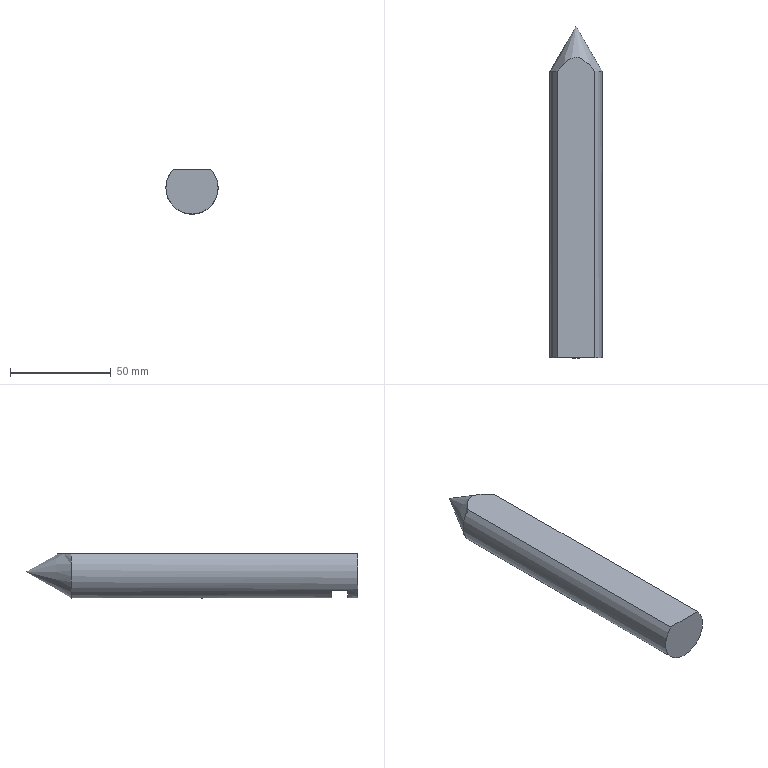Part | NX | features EXTRUDE 4, DATUM_CSYS 2, CONE 1, DATUM_PLANE 1, RECT_SLOT 1, SKETCH 1 | 1 solid | 12 faces | box 26 x 165 x 22 mm | volume 69817 mm3 | plane 7 | cylinder 4 | cone 1 | commonest cylinder face diameters 5 x2 26 x1 32 x1
STEP:
#1=CARTESIAN_POINT('',(-9.381,142.483,9.));
#2=VERTEX_POINT('',#1);
#3=CARTESIAN_POINT('',(0.06208,142.483,-13.));
#4=VERTEX_POINT('',#3);
#5=CARTESIAN_POINT('',(0.,142.483,0.));
#6=DIRECTION('',(0.,-1.,0.));
#7=DIRECTION('',(0.,0.,-1.));
#8=AXIS2_PLACEMENT_3D('',#5,#6,#7);
#9=CIRCLE('',#8,13.);
#10=EDGE_CURVE('',#2,#4,#9,.T.);
#11=ORIENTED_EDGE('',*,*,#10,.T.);
#12=CARTESIAN_POINT('',(-2.438,139.983,-12.769));
#13=VERTEX_POINT('',#12);
#14=CARTESIAN_POINT('',(0.06208,142.483,-13.));
#15=CARTESIAN_POINT('',(-0.5912,142.483,-13.003));
#16=CARTESIAN_POINT('',(-1.896,141.938,-12.889));
#17=CARTESIAN_POINT('',(-2.438,140.645,-12.769));
#18=CARTESIAN_POINT('',(-2.438,139.983,-12.769));
#19=B_SPLINE_CURVE_WITH_KNOTS('',3,(#14,#15,#16,#17,#18),.UNSPECIFIED.,.F.,.F.,(4,1,4),(0.003919,0.005876,0.007832),.UNSPECIFIED.);
#20=EDGE_CURVE('',#4,#13,#19,.T.);
#21=ORIENTED_EDGE('',*,*,#20,.T.);
#22=CARTESIAN_POINT('',(-2.438,79.983,-12.769));
#23=VERTEX_POINT('',#22);
#24=CARTESIAN_POINT('',(-2.438,140.,-12.769));
#25=DIRECTION('',(0.,-1.,0.));
#26=VECTOR('',#25,1000.);
#27=LINE('',#24,#26);
#28=EDGE_CURVE('',#13,#23,#27,.T.);
#29=ORIENTED_EDGE('',*,*,#28,.T.);
#30=CARTESIAN_POINT('',(2.562,79.983,-12.745));
#31=VERTEX_POINT('',#30);
#32=CARTESIAN_POINT('',(-2.438,79.983,-12.769));
#33=CARTESIAN_POINT('',(-2.438,79.321,-12.769));
#34=CARTESIAN_POINT('',(-1.896,78.028,-12.889));
#35=CARTESIAN_POINT('',(0.06023,77.211,-13.06));
#36=CARTESIAN_POINT('',(2.02,78.028,-12.87));
#37=CARTESIAN_POINT('',(2.562,79.321,-12.745));
#38=CARTESIAN_POINT('',(2.562,79.983,-12.745));
#39=B_SPLINE_CURVE_WITH_KNOTS('',3,(#32,#33,#34,#35,#36,#37,#38),.UNSPECIFIED.,.F.,.F.,(4,1,1,1,4),(0.,0.001958,0.003916,0.005874,0.007832),.UNSPECIFIED.);
#40=EDGE_CURVE('',#23,#31,#39,.T.);
#41=ORIENTED_EDGE('',*,*,#40,.T.);
#42=CARTESIAN_POINT('',(2.562,139.983,-12.745));
#43=VERTEX_POINT('',#42);
#44=CARTESIAN_POINT('',(2.562,140.,-12.745));
#45=DIRECTION('',(0.,-1.,0.));
#46=VECTOR('',#45,1000.);
#47=LINE('',#44,#46);
#48=EDGE_CURVE('',#31,#43,#47,.F.);
#49=ORIENTED_EDGE('',*,*,#48,.T.);
#50=CARTESIAN_POINT('',(2.562,139.983,-12.745));
#51=CARTESIAN_POINT('',(2.562,140.646,-12.745));
#52=CARTESIAN_POINT('',(2.019,141.939,-12.87));
#53=CARTESIAN_POINT('',(0.7163,142.483,-12.997));
#54=CARTESIAN_POINT('',(0.06208,142.483,-13.));
#55=B_SPLINE_CURVE_WITH_KNOTS('',3,(#50,#51,#52,#53,#54),.UNSPECIFIED.,.F.,.F.,(4,1,4),(0.,0.001959,0.003919),.UNSPECIFIED.);
#56=EDGE_CURVE('',#43,#4,#55,.T.);
#57=ORIENTED_EDGE('',*,*,#56,.T.);
#58=CARTESIAN_POINT('',(9.381,142.483,9.));
#59=VERTEX_POINT('',#58);
#60=CARTESIAN_POINT('',(0.,142.483,0.));
#61=DIRECTION('',(0.,-1.,0.));
#62=DIRECTION('',(0.,0.,-1.));
#63=AXIS2_PLACEMENT_3D('',#60,#61,#62);
#64=CIRCLE('',#63,13.);
#65=EDGE_CURVE('',#4,#59,#64,.T.);
#66=ORIENTED_EDGE('',*,*,#65,.T.);
#67=CARTESIAN_POINT('',(9.381,0.,9.));
#68=VERTEX_POINT('',#67);
#69=CARTESIAN_POINT('',(9.381,140.,9.));
#70=DIRECTION('',(0.,-1.,0.));
#71=VECTOR('',#70,1000.);
#72=LINE('',#69,#71);
#73=EDGE_CURVE('',#68,#59,#72,.F.);
#74=ORIENTED_EDGE('',*,*,#73,.F.);
#75=CARTESIAN_POINT('',(-9.381,0.,9.));
#76=VERTEX_POINT('',#75);
#77=CARTESIAN_POINT('',(0.,0.,0.));
#78=DIRECTION('',(0.,1.,0.));
#79=DIRECTION('',(1.,0.,0.));
#80=AXIS2_PLACEMENT_3D('',#77,#78,#79);
#81=CIRCLE('',#80,13.);
#82=EDGE_CURVE('',#68,#76,#81,.T.);
#83=ORIENTED_EDGE('',*,*,#82,.T.);
#84=CARTESIAN_POINT('',(-9.381,140.,9.));
#85=DIRECTION('',(0.,-1.,0.));
#86=VECTOR('',#85,1000.);
#87=LINE('',#84,#86);
#88=EDGE_CURVE('',#2,#76,#87,.T.);
#89=ORIENTED_EDGE('',*,*,#88,.F.);
#90=EDGE_LOOP('',(#11,#21,#29,#41,#49,#57,#66,#74,#83,#89));
#91=FACE_BOUND('',#90,.T.);
#92=CARTESIAN_POINT('',(-9.381,13.,-9.));
#93=VERTEX_POINT('',#92);
#94=CARTESIAN_POINT('',(9.381,13.,-9.));
#95=VERTEX_POINT('',#94);
#96=CARTESIAN_POINT('',(0.,13.,0.));
#97=DIRECTION('',(0.,-1.,0.));
#98=DIRECTION('',(0.,0.,-1.));
#99=AXIS2_PLACEMENT_3D('',#96,#97,#98);
#100=CIRCLE('',#99,13.);
#101=EDGE_CURVE('',#93,#95,#100,.T.);
#102=ORIENTED_EDGE('',*,*,#101,.F.);
#103=CARTESIAN_POINT('',(-9.381,5.,-9.));
#104=VERTEX_POINT('',#103);
#105=CARTESIAN_POINT('',(-9.381,9.,-9.));
#106=DIRECTION('',(0.,-1.,0.));
#107=VECTOR('',#106,1000.);
#108=LINE('',#105,#107);
#109=EDGE_CURVE('',#93,#104,#108,.T.);
#110=ORIENTED_EDGE('',*,*,#109,.T.);
#111=CARTESIAN_POINT('',(9.381,5.,-9.));
#112=VERTEX_POINT('',#111);
#113=CARTESIAN_POINT('',(0.,5.,0.));
#114=DIRECTION('',(0.,-1.,0.));
#115=DIRECTION('',(0.,0.,-1.));
#116=AXIS2_PLACEMENT_3D('',#113,#114,#115);
#117=CIRCLE('',#116,13.);
#118=EDGE_CURVE('',#104,#112,#117,.T.);
#119=ORIENTED_EDGE('',*,*,#118,.T.);
#120=CARTESIAN_POINT('',(9.381,9.,-9.));
#121=DIRECTION('',(0.,-1.,0.));
#122=VECTOR('',#121,1000.);
#123=LINE('',#120,#122);
#124=EDGE_CURVE('',#112,#95,#123,.F.);
#125=ORIENTED_EDGE('',*,*,#124,.T.);
#126=EDGE_LOOP('',(#102,#110,#119,#125));
#127=FACE_BOUND('',#126,.T.);
#128=CARTESIAN_POINT('',(0.,140.,0.));
#129=DIRECTION('',(0.,-1.,0.));
#130=DIRECTION('',(0.,0.,-1.));
#131=AXIS2_PLACEMENT_3D('',#128,#129,#130);
#132=CYLINDRICAL_SURFACE('',#131,13.);
#133=ADVANCED_FACE('',(#91,#127),#132,.T.);
#134=CARTESIAN_POINT('',(0.,165.,0.));
#135=VERTEX_POINT('',#134);
#136=VERTEX_LOOP('',#135);
#137=FACE_BOUND('',#136,.T.);
#138=ORIENTED_EDGE('',*,*,#10,.F.);
#139=CARTESIAN_POINT('',(-9.381,142.483,9.));
#140=CARTESIAN_POINT('',(-8.755,143.266,9.));
#141=CARTESIAN_POINT('',(-7.465,144.807,9.));
#142=CARTESIAN_POINT('',(-5.351,146.958,9.));
#143=CARTESIAN_POINT('',(-2.95,148.801,9.));
#144=CARTESIAN_POINT('',(0.04464,149.726,9.));
#145=CARTESIAN_POINT('',(3.007,148.764,9.));
#146=CARTESIAN_POINT('',(5.399,146.914,9.));
#147=CARTESIAN_POINT('',(7.477,144.792,9.));
#148=CARTESIAN_POINT('',(8.758,143.262,9.));
#149=CARTESIAN_POINT('',(9.381,142.483,9.));
#150=B_SPLINE_CURVE_WITH_KNOTS('',3,(#139,#140,#141,#142,#143,#144,#145,#146,#147,#148,#149),.UNSPECIFIED.,.F.,.F.,(4,1,1,1,1,1,1,1,4),(0.0127,0.0157,0.0187,0.0217,0.02471,0.02771,0.03071,0.03372,0.03672),.UNSPECIFIED.);
#151=EDGE_CURVE('',#2,#59,#150,.T.);
#152=ORIENTED_EDGE('',*,*,#151,.T.);
#153=ORIENTED_EDGE('',*,*,#65,.F.);
#154=EDGE_LOOP('',(#138,#152,#153));
#155=FACE_BOUND('',#154,.T.);
#156=CARTESIAN_POINT('',(0.,165.,0.));
#157=DIRECTION('',(0.,-1.,0.));
#158=DIRECTION('',(1.,0.,0.));
#159=AXIS2_PLACEMENT_3D('',#156,#157,#158);
#160=CONICAL_SURFACE('',#159,0.,0.5236);
#161=ADVANCED_FACE('',(#137,#155),#160,.T.);
#162=CARTESIAN_POINT('',(-9.381,0.,9.));
#163=DIRECTION('',(1.,0.,0.));
#164=VECTOR('',#163,1000.);
#165=LINE('',#162,#164);
#166=EDGE_CURVE('',#76,#68,#165,.T.);
#167=ORIENTED_EDGE('',*,*,#166,.T.);
#168=ORIENTED_EDGE('',*,*,#73,.T.);
#169=ORIENTED_EDGE('',*,*,#151,.F.);
#170=ORIENTED_EDGE('',*,*,#88,.T.);
#171=EDGE_LOOP('',(#167,#168,#169,#170));
#172=FACE_BOUND('',#171,.T.);
#173=CARTESIAN_POINT('',(-9.381,140.,9.));
#174=DIRECTION('',(0.,0.,-1.));
#175=DIRECTION('',(-1.,0.,0.));
#176=AXIS2_PLACEMENT_3D('',#173,#174,#175);
#177=PLANE('',#176);
#178=ADVANCED_FACE('',(#172),#177,.F.);
#179=ORIENTED_EDGE('',*,*,#82,.F.);
#180=ORIENTED_EDGE('',*,*,#166,.F.);
#181=EDGE_LOOP('',(#179,#180));
#182=FACE_BOUND('',#181,.T.);
#183=CARTESIAN_POINT('',(0.,0.,0.));
#184=DIRECTION('',(0.,1.,0.));
#185=DIRECTION('',(0.,0.,1.));
#186=AXIS2_PLACEMENT_3D('',#183,#184,#185);
#187=PLANE('',#186);
#188=ADVANCED_FACE('',(#182),#187,.F.);
#189=CARTESIAN_POINT('',(0.,5.,-21.961));
#190=DIRECTION('',(0.,-1.,0.));
#191=DIRECTION('',(1.,0.,0.));
#192=AXIS2_PLACEMENT_3D('',#189,#190,#191);
#193=CIRCLE('',#192,16.);
#194=EDGE_CURVE('',#104,#112,#193,.F.);
#195=ORIENTED_EDGE('',*,*,#194,.F.);
#196=ORIENTED_EDGE('',*,*,#109,.F.);
#197=CARTESIAN_POINT('',(0.,13.,-21.961));
#198=DIRECTION('',(0.,-1.,0.));
#199=DIRECTION('',(1.,0.,0.));
#200=AXIS2_PLACEMENT_3D('',#197,#198,#199);
#201=CIRCLE('',#200,16.);
#202=EDGE_CURVE('',#93,#95,#201,.F.);
#203=ORIENTED_EDGE('',*,*,#202,.T.);
#204=ORIENTED_EDGE('',*,*,#124,.F.);
#205=EDGE_LOOP('',(#195,#196,#203,#204));
#206=FACE_BOUND('',#205,.T.);
#207=CARTESIAN_POINT('',(0.,13.,-21.961));
#208=DIRECTION('',(0.,-1.,0.));
#209=DIRECTION('',(0.,0.,-1.));
#210=AXIS2_PLACEMENT_3D('',#207,#208,#209);
#211=CYLINDRICAL_SURFACE('',#210,16.);
#212=ADVANCED_FACE('',(#206),#211,.F.);
#213=ORIENTED_EDGE('',*,*,#101,.T.);
#214=ORIENTED_EDGE('',*,*,#202,.F.);
#215=EDGE_LOOP('',(#213,#214));
#216=FACE_BOUND('',#215,.T.);
#217=CARTESIAN_POINT('',(0.,13.,-21.961));
#218=DIRECTION('',(0.,-1.,0.));
#219=DIRECTION('',(0.,0.,-1.));
#220=AXIS2_PLACEMENT_3D('',#217,#218,#219);
#221=PLANE('',#220);
#222=ADVANCED_FACE('',(#216),#221,.T.);
#223=ORIENTED_EDGE('',*,*,#194,.T.);
#224=ORIENTED_EDGE('',*,*,#118,.F.);
#225=EDGE_LOOP('',(#223,#224));
#226=FACE_BOUND('',#225,.T.);
#227=CARTESIAN_POINT('',(0.,5.,-21.961));
#228=DIRECTION('',(0.,-1.,0.));
#229=DIRECTION('',(0.,0.,-1.));
#230=AXIS2_PLACEMENT_3D('',#227,#228,#229);
#231=PLANE('',#230);
#232=ADVANCED_FACE('',(#226),#231,.F.);
#233=CARTESIAN_POINT('',(-2.438,139.983,-8.));
#234=VERTEX_POINT('',#233);
#235=CARTESIAN_POINT('',(-2.438,139.983,-13.));
#236=DIRECTION('',(0.,0.,-1.));
#237=VECTOR('',#236,1000.);
#238=LINE('',#235,#237);
#239=EDGE_CURVE('',#13,#234,#238,.F.);
#240=ORIENTED_EDGE('',*,*,#239,.T.);
#241=CARTESIAN_POINT('',(-2.438,79.983,-8.));
#242=VERTEX_POINT('',#241);
#243=CARTESIAN_POINT('',(-2.438,139.983,-8.));
#244=DIRECTION('',(0.,-1.,0.));
#245=VECTOR('',#244,1000.);
#246=LINE('',#243,#245);
#247=EDGE_CURVE('',#242,#234,#246,.F.);
#248=ORIENTED_EDGE('',*,*,#247,.F.);
#249=CARTESIAN_POINT('',(-2.438,79.983,-13.));
#250=DIRECTION('',(0.,0.,-1.));
#251=VECTOR('',#250,1000.);
#252=LINE('',#249,#251);
#253=EDGE_CURVE('',#23,#242,#252,.F.);
#254=ORIENTED_EDGE('',*,*,#253,.F.);
#255=ORIENTED_EDGE('',*,*,#28,.F.);
#256=EDGE_LOOP('',(#240,#248,#254,#255));
#257=FACE_BOUND('',#256,.T.);
#258=CARTESIAN_POINT('',(-2.438,109.983,-13.));
#259=DIRECTION('',(-1.,0.,0.));
#260=DIRECTION('',(0.,0.,1.));
#261=AXIS2_PLACEMENT_3D('',#258,#259,#260);
#262=PLANE('',#261);
#263=ADVANCED_FACE('',(#257),#262,.F.);
#264=CARTESIAN_POINT('',(2.562,79.983,-8.));
#265=VERTEX_POINT('',#264);
#266=CARTESIAN_POINT('',(2.562,79.983,-13.));
#267=DIRECTION('',(0.,0.,-1.));
#268=VECTOR('',#267,1000.);
#269=LINE('',#266,#268);
#270=EDGE_CURVE('',#31,#265,#269,.F.);
#271=ORIENTED_EDGE('',*,*,#270,.T.);
#272=CARTESIAN_POINT('',(2.562,139.983,-8.));
#273=VERTEX_POINT('',#272);
#274=CARTESIAN_POINT('',(2.562,139.983,-8.));
#275=DIRECTION('',(0.,-1.,0.));
#276=VECTOR('',#275,1000.);
#277=LINE('',#274,#276);
#278=EDGE_CURVE('',#265,#273,#277,.F.);
#279=ORIENTED_EDGE('',*,*,#278,.T.);
#280=CARTESIAN_POINT('',(2.562,139.983,-13.));
#281=DIRECTION('',(0.,0.,-1.));
#282=VECTOR('',#281,1000.);
#283=LINE('',#280,#282);
#284=EDGE_CURVE('',#43,#273,#283,.F.);
#285=ORIENTED_EDGE('',*,*,#284,.F.);
#286=ORIENTED_EDGE('',*,*,#48,.F.);
#287=EDGE_LOOP('',(#271,#279,#285,#286));
#288=FACE_BOUND('',#287,.T.);
#289=CARTESIAN_POINT('',(2.562,109.983,-13.));
#290=DIRECTION('',(1.,0.,0.));
#291=DIRECTION('',(0.,0.,-1.));
#292=AXIS2_PLACEMENT_3D('',#289,#290,#291);
#293=PLANE('',#292);
#294=ADVANCED_FACE('',(#288),#293,.F.);
#295=ORIENTED_EDGE('',*,*,#253,.T.);
#296=CARTESIAN_POINT('',(0.06208,79.983,-8.));
#297=DIRECTION('',(0.,0.,-1.));
#298=DIRECTION('',(-1.,0.,0.));
#299=AXIS2_PLACEMENT_3D('',#296,#297,#298);
#300=CIRCLE('',#299,2.5);
#301=EDGE_CURVE('',#242,#265,#300,.F.);
#302=ORIENTED_EDGE('',*,*,#301,.T.);
#303=ORIENTED_EDGE('',*,*,#270,.F.);
#304=ORIENTED_EDGE('',*,*,#40,.F.);
#305=EDGE_LOOP('',(#295,#302,#303,#304));
#306=FACE_BOUND('',#305,.T.);
#307=CARTESIAN_POINT('',(0.06208,79.983,-13.));
#308=DIRECTION('',(0.,0.,-1.));
#309=DIRECTION('',(-1.,0.,0.));
#310=AXIS2_PLACEMENT_3D('',#307,#308,#309);
#311=CYLINDRICAL_SURFACE('',#310,2.5);
#312=ADVANCED_FACE('',(#306),#311,.F.);
#313=ORIENTED_EDGE('',*,*,#284,.T.);
#314=CARTESIAN_POINT('',(0.06208,139.983,-8.));
#315=DIRECTION('',(0.,0.,-1.));
#316=DIRECTION('',(-1.,0.,0.));
#317=AXIS2_PLACEMENT_3D('',#314,#315,#316);
#318=CIRCLE('',#317,2.5);
#319=EDGE_CURVE('',#273,#234,#318,.F.);
#320=ORIENTED_EDGE('',*,*,#319,.T.);
#321=ORIENTED_EDGE('',*,*,#239,.F.);
#322=ORIENTED_EDGE('',*,*,#20,.F.);
#323=ORIENTED_EDGE('',*,*,#56,.F.);
#324=EDGE_LOOP('',(#313,#320,#321,#322,#323));
#325=FACE_BOUND('',#324,.T.);
#326=CARTESIAN_POINT('',(0.06208,139.983,-13.));
#327=DIRECTION('',(0.,0.,-1.));
#328=DIRECTION('',(-1.,0.,0.));
#329=AXIS2_PLACEMENT_3D('',#326,#327,#328);
#330=CYLINDRICAL_SURFACE('',#329,2.5);
#331=ADVANCED_FACE('',(#325),#330,.F.);
#332=ORIENTED_EDGE('',*,*,#247,.T.);
#333=ORIENTED_EDGE('',*,*,#319,.F.);
#334=ORIENTED_EDGE('',*,*,#278,.F.);
#335=ORIENTED_EDGE('',*,*,#301,.F.);
#336=EDGE_LOOP('',(#332,#333,#334,#335));
#337=FACE_BOUND('',#336,.T.);
#338=CARTESIAN_POINT('',(0.06208,109.983,-8.));
#339=DIRECTION('',(0.,0.,1.));
#340=DIRECTION('',(1.,0.,0.));
#341=AXIS2_PLACEMENT_3D('',#338,#339,#340);
#342=PLANE('',#341);
#343=ADVANCED_FACE('',(#337),#342,.F.);
#344=CLOSED_SHELL('',(#133,#161,#178,#188,#212,#222,#232,#263,#294,#312,#331,#343));
#345=MANIFOLD_SOLID_BREP('',#344);
#346=(LENGTH_UNIT()NAMED_UNIT(*)SI_UNIT(.MILLI.,.METRE.));
#347=UNCERTAINTY_MEASURE_WITH_UNIT(LENGTH_MEASURE(0.0508),#346,'','');
#348=(NAMED_UNIT(*)PLANE_ANGLE_UNIT()SI_UNIT($,.RADIAN.));
#349=(NAMED_UNIT(*)SI_UNIT($,.STERADIAN.)SOLID_ANGLE_UNIT());
#350=(GEOMETRIC_REPRESENTATION_CONTEXT(3)GLOBAL_UNCERTAINTY_ASSIGNED_CONTEXT((#347))GLOBAL_UNIT_ASSIGNED_CONTEXT((#346,#348,#349))REPRESENTATION_CONTEXT('',''));
#351=ADVANCED_BREP_SHAPE_REPRESENTATION('',(#345),#350);